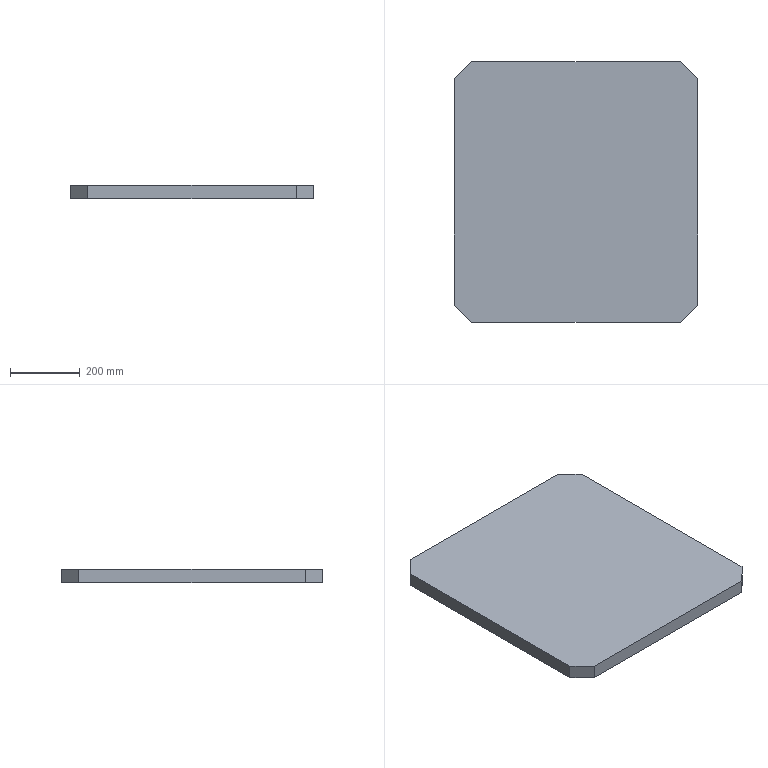Part | SolidWorks | features Extrusion 1 | 1 solid | 10 faces | box 700 x 750 x 40 mm | volume 20800000 mm3 | plane 10
STEP:
#1=CARTESIAN_POINT('',(650.,750.,0.));
#2=VERTEX_POINT('',#1);
#3=CARTESIAN_POINT('',(50.,750.,0.));
#4=VERTEX_POINT('',#3);
#5=CARTESIAN_POINT('',(50.,750.,0.));
#6=DIRECTION('',(-1.,0.,0.));
#7=VECTOR('',#6,1000.);
#8=LINE('',#5,#7);
#9=EDGE_CURVE('',#2,#4,#8,.T.);
#10=ORIENTED_EDGE('',*,*,#9,.T.);
#11=CARTESIAN_POINT('',(50.,750.,40.));
#12=VERTEX_POINT('',#11);
#13=CARTESIAN_POINT('',(50.,750.,40.));
#14=DIRECTION('',(0.,0.,-1.));
#15=VECTOR('',#14,1000.);
#16=LINE('',#13,#15);
#17=EDGE_CURVE('',#12,#4,#16,.T.);
#18=ORIENTED_EDGE('',*,*,#17,.F.);
#19=CARTESIAN_POINT('',(650.,750.,40.));
#20=VERTEX_POINT('',#19);
#21=CARTESIAN_POINT('',(50.,750.,40.));
#22=DIRECTION('',(-1.,0.,0.));
#23=VECTOR('',#22,1000.);
#24=LINE('',#21,#23);
#25=EDGE_CURVE('',#20,#12,#24,.T.);
#26=ORIENTED_EDGE('',*,*,#25,.F.);
#27=CARTESIAN_POINT('',(650.,750.,40.));
#28=DIRECTION('',(0.,0.,-1.));
#29=VECTOR('',#28,1000.);
#30=LINE('',#27,#29);
#31=EDGE_CURVE('',#20,#2,#30,.T.);
#32=ORIENTED_EDGE('',*,*,#31,.T.);
#33=EDGE_LOOP('',(#10,#18,#26,#32));
#34=FACE_OUTER_BOUND('',#33,.T.);
#35=CARTESIAN_POINT('',(50.,750.,40.));
#36=DIRECTION('',(0.,-1.,0.));
#37=DIRECTION('',(0.,0.,-1.));
#38=AXIS2_PLACEMENT_3D('',#35,#36,#37);
#39=PLANE('',#38);
#40=ADVANCED_FACE('',(#34),#39,.F.);
#41=CARTESIAN_POINT('',(0.,700.,0.));
#42=VERTEX_POINT('',#41);
#43=CARTESIAN_POINT('',(0.,700.,0.));
#44=DIRECTION('',(-0.7071,-0.7071,0.));
#45=VECTOR('',#44,1000.);
#46=LINE('',#43,#45);
#47=EDGE_CURVE('',#4,#42,#46,.T.);
#48=ORIENTED_EDGE('',*,*,#47,.T.);
#49=CARTESIAN_POINT('',(0.,700.,40.));
#50=VERTEX_POINT('',#49);
#51=CARTESIAN_POINT('',(0.,700.,40.));
#52=DIRECTION('',(0.,0.,-1.));
#53=VECTOR('',#52,1000.);
#54=LINE('',#51,#53);
#55=EDGE_CURVE('',#50,#42,#54,.T.);
#56=ORIENTED_EDGE('',*,*,#55,.F.);
#57=CARTESIAN_POINT('',(0.,700.,40.));
#58=DIRECTION('',(-0.7071,-0.7071,0.));
#59=VECTOR('',#58,1000.);
#60=LINE('',#57,#59);
#61=EDGE_CURVE('',#12,#50,#60,.T.);
#62=ORIENTED_EDGE('',*,*,#61,.F.);
#63=ORIENTED_EDGE('',*,*,#17,.T.);
#64=EDGE_LOOP('',(#48,#56,#62,#63));
#65=FACE_OUTER_BOUND('',#64,.T.);
#66=CARTESIAN_POINT('',(0.,700.,40.));
#67=DIRECTION('',(0.7071,-0.7071,0.));
#68=DIRECTION('',(0.7071,0.7071,0.));
#69=AXIS2_PLACEMENT_3D('',#66,#67,#68);
#70=PLANE('',#69);
#71=ADVANCED_FACE('',(#65),#70,.F.);
#72=CARTESIAN_POINT('',(0.,50.,0.));
#73=VERTEX_POINT('',#72);
#74=CARTESIAN_POINT('',(0.,50.,0.));
#75=DIRECTION('',(0.,-1.,0.));
#76=VECTOR('',#75,1000.);
#77=LINE('',#74,#76);
#78=EDGE_CURVE('',#42,#73,#77,.T.);
#79=ORIENTED_EDGE('',*,*,#78,.T.);
#80=CARTESIAN_POINT('',(0.,50.,40.));
#81=VERTEX_POINT('',#80);
#82=CARTESIAN_POINT('',(0.,50.,40.));
#83=DIRECTION('',(0.,0.,-1.));
#84=VECTOR('',#83,1000.);
#85=LINE('',#82,#84);
#86=EDGE_CURVE('',#81,#73,#85,.T.);
#87=ORIENTED_EDGE('',*,*,#86,.F.);
#88=CARTESIAN_POINT('',(0.,50.,40.));
#89=DIRECTION('',(0.,-1.,0.));
#90=VECTOR('',#89,1000.);
#91=LINE('',#88,#90);
#92=EDGE_CURVE('',#50,#81,#91,.T.);
#93=ORIENTED_EDGE('',*,*,#92,.F.);
#94=ORIENTED_EDGE('',*,*,#55,.T.);
#95=EDGE_LOOP('',(#79,#87,#93,#94));
#96=FACE_OUTER_BOUND('',#95,.T.);
#97=CARTESIAN_POINT('',(0.,50.,40.));
#98=DIRECTION('',(1.,0.,0.));
#99=DIRECTION('',(0.,0.,-1.));
#100=AXIS2_PLACEMENT_3D('',#97,#98,#99);
#101=PLANE('',#100);
#102=ADVANCED_FACE('',(#96),#101,.F.);
#103=CARTESIAN_POINT('',(50.,0.,0.));
#104=VERTEX_POINT('',#103);
#105=CARTESIAN_POINT('',(50.,0.,0.));
#106=DIRECTION('',(0.7071,-0.7071,0.));
#107=VECTOR('',#106,1000.);
#108=LINE('',#105,#107);
#109=EDGE_CURVE('',#73,#104,#108,.T.);
#110=ORIENTED_EDGE('',*,*,#109,.T.);
#111=CARTESIAN_POINT('',(50.,0.,40.));
#112=VERTEX_POINT('',#111);
#113=CARTESIAN_POINT('',(50.,0.,40.));
#114=DIRECTION('',(0.,0.,-1.));
#115=VECTOR('',#114,1000.);
#116=LINE('',#113,#115);
#117=EDGE_CURVE('',#112,#104,#116,.T.);
#118=ORIENTED_EDGE('',*,*,#117,.F.);
#119=CARTESIAN_POINT('',(50.,0.,40.));
#120=DIRECTION('',(0.7071,-0.7071,0.));
#121=VECTOR('',#120,1000.);
#122=LINE('',#119,#121);
#123=EDGE_CURVE('',#81,#112,#122,.T.);
#124=ORIENTED_EDGE('',*,*,#123,.F.);
#125=ORIENTED_EDGE('',*,*,#86,.T.);
#126=EDGE_LOOP('',(#110,#118,#124,#125));
#127=FACE_OUTER_BOUND('',#126,.T.);
#128=CARTESIAN_POINT('',(50.,0.,40.));
#129=DIRECTION('',(0.7071,0.7071,0.));
#130=DIRECTION('',(-0.7071,0.7071,0.));
#131=AXIS2_PLACEMENT_3D('',#128,#129,#130);
#132=PLANE('',#131);
#133=ADVANCED_FACE('',(#127),#132,.F.);
#134=CARTESIAN_POINT('',(650.,0.,0.));
#135=VERTEX_POINT('',#134);
#136=CARTESIAN_POINT('',(50.,0.,0.));
#137=DIRECTION('',(1.,0.,0.));
#138=VECTOR('',#137,1000.);
#139=LINE('',#136,#138);
#140=EDGE_CURVE('',#104,#135,#139,.T.);
#141=ORIENTED_EDGE('',*,*,#140,.T.);
#142=CARTESIAN_POINT('',(650.,0.,40.));
#143=VERTEX_POINT('',#142);
#144=CARTESIAN_POINT('',(650.,0.,40.));
#145=DIRECTION('',(0.,0.,-1.));
#146=VECTOR('',#145,1000.);
#147=LINE('',#144,#146);
#148=EDGE_CURVE('',#143,#135,#147,.T.);
#149=ORIENTED_EDGE('',*,*,#148,.F.);
#150=CARTESIAN_POINT('',(50.,0.,40.));
#151=DIRECTION('',(1.,0.,0.));
#152=VECTOR('',#151,1000.);
#153=LINE('',#150,#152);
#154=EDGE_CURVE('',#112,#143,#153,.T.);
#155=ORIENTED_EDGE('',*,*,#154,.F.);
#156=ORIENTED_EDGE('',*,*,#117,.T.);
#157=EDGE_LOOP('',(#141,#149,#155,#156));
#158=FACE_OUTER_BOUND('',#157,.T.);
#159=CARTESIAN_POINT('',(50.,0.,40.));
#160=DIRECTION('',(0.,1.,0.));
#161=DIRECTION('',(0.,0.,1.));
#162=AXIS2_PLACEMENT_3D('',#159,#160,#161);
#163=PLANE('',#162);
#164=ADVANCED_FACE('',(#158),#163,.F.);
#165=CARTESIAN_POINT('',(700.,50.,0.));
#166=VERTEX_POINT('',#165);
#167=CARTESIAN_POINT('',(650.,0.,0.));
#168=DIRECTION('',(0.7071,0.7071,0.));
#169=VECTOR('',#168,1000.);
#170=LINE('',#167,#169);
#171=EDGE_CURVE('',#135,#166,#170,.T.);
#172=ORIENTED_EDGE('',*,*,#171,.T.);
#173=CARTESIAN_POINT('',(700.,50.,40.));
#174=VERTEX_POINT('',#173);
#175=CARTESIAN_POINT('',(700.,50.,40.));
#176=DIRECTION('',(0.,0.,-1.));
#177=VECTOR('',#176,1000.);
#178=LINE('',#175,#177);
#179=EDGE_CURVE('',#174,#166,#178,.T.);
#180=ORIENTED_EDGE('',*,*,#179,.F.);
#181=CARTESIAN_POINT('',(650.,0.,40.));
#182=DIRECTION('',(0.7071,0.7071,0.));
#183=VECTOR('',#182,1000.);
#184=LINE('',#181,#183);
#185=EDGE_CURVE('',#143,#174,#184,.T.);
#186=ORIENTED_EDGE('',*,*,#185,.F.);
#187=ORIENTED_EDGE('',*,*,#148,.T.);
#188=EDGE_LOOP('',(#172,#180,#186,#187));
#189=FACE_OUTER_BOUND('',#188,.T.);
#190=CARTESIAN_POINT('',(650.,0.,40.));
#191=DIRECTION('',(-0.7071,0.7071,0.));
#192=DIRECTION('',(-0.7071,-0.7071,0.));
#193=AXIS2_PLACEMENT_3D('',#190,#191,#192);
#194=PLANE('',#193);
#195=ADVANCED_FACE('',(#189),#194,.F.);
#196=CARTESIAN_POINT('',(700.,700.,0.));
#197=VERTEX_POINT('',#196);
#198=CARTESIAN_POINT('',(700.,50.,0.));
#199=DIRECTION('',(0.,1.,0.));
#200=VECTOR('',#199,1000.);
#201=LINE('',#198,#200);
#202=EDGE_CURVE('',#166,#197,#201,.T.);
#203=ORIENTED_EDGE('',*,*,#202,.T.);
#204=CARTESIAN_POINT('',(700.,700.,40.));
#205=VERTEX_POINT('',#204);
#206=CARTESIAN_POINT('',(700.,700.,40.));
#207=DIRECTION('',(0.,0.,-1.));
#208=VECTOR('',#207,1000.);
#209=LINE('',#206,#208);
#210=EDGE_CURVE('',#205,#197,#209,.T.);
#211=ORIENTED_EDGE('',*,*,#210,.F.);
#212=CARTESIAN_POINT('',(700.,50.,40.));
#213=DIRECTION('',(0.,1.,0.));
#214=VECTOR('',#213,1000.);
#215=LINE('',#212,#214);
#216=EDGE_CURVE('',#174,#205,#215,.T.);
#217=ORIENTED_EDGE('',*,*,#216,.F.);
#218=ORIENTED_EDGE('',*,*,#179,.T.);
#219=EDGE_LOOP('',(#203,#211,#217,#218));
#220=FACE_OUTER_BOUND('',#219,.T.);
#221=CARTESIAN_POINT('',(700.,50.,40.));
#222=DIRECTION('',(-1.,0.,0.));
#223=DIRECTION('',(0.,0.,1.));
#224=AXIS2_PLACEMENT_3D('',#221,#222,#223);
#225=PLANE('',#224);
#226=ADVANCED_FACE('',(#220),#225,.F.);
#227=CARTESIAN_POINT('',(650.,750.,0.));
#228=DIRECTION('',(-0.7071,0.7071,0.));
#229=VECTOR('',#228,1000.);
#230=LINE('',#227,#229);
#231=EDGE_CURVE('',#197,#2,#230,.T.);
#232=ORIENTED_EDGE('',*,*,#231,.T.);
#233=ORIENTED_EDGE('',*,*,#31,.F.);
#234=CARTESIAN_POINT('',(650.,750.,40.));
#235=DIRECTION('',(-0.7071,0.7071,0.));
#236=VECTOR('',#235,1000.);
#237=LINE('',#234,#236);
#238=EDGE_CURVE('',#205,#20,#237,.T.);
#239=ORIENTED_EDGE('',*,*,#238,.F.);
#240=ORIENTED_EDGE('',*,*,#210,.T.);
#241=EDGE_LOOP('',(#232,#233,#239,#240));
#242=FACE_OUTER_BOUND('',#241,.T.);
#243=CARTESIAN_POINT('',(650.,750.,40.));
#244=DIRECTION('',(-0.7071,-0.7071,0.));
#245=DIRECTION('',(0.7071,-0.7071,0.));
#246=AXIS2_PLACEMENT_3D('',#243,#244,#245);
#247=PLANE('',#246);
#248=ADVANCED_FACE('',(#242),#247,.F.);
#249=ORIENTED_EDGE('',*,*,#25,.T.);
#250=ORIENTED_EDGE('',*,*,#61,.T.);
#251=ORIENTED_EDGE('',*,*,#92,.T.);
#252=ORIENTED_EDGE('',*,*,#123,.T.);
#253=ORIENTED_EDGE('',*,*,#154,.T.);
#254=ORIENTED_EDGE('',*,*,#185,.T.);
#255=ORIENTED_EDGE('',*,*,#216,.T.);
#256=ORIENTED_EDGE('',*,*,#238,.T.);
#257=EDGE_LOOP('',(#249,#250,#251,#252,#253,#254,#255,#256));
#258=FACE_OUTER_BOUND('',#257,.T.);
#259=CARTESIAN_POINT('',(700.,750.,40.));
#260=DIRECTION('',(0.,0.,1.));
#261=DIRECTION('',(1.,0.,0.));
#262=AXIS2_PLACEMENT_3D('',#259,#260,#261);
#263=PLANE('',#262);
#264=ADVANCED_FACE('',(#258),#263,.T.);
#265=ORIENTED_EDGE('',*,*,#9,.F.);
#266=ORIENTED_EDGE('',*,*,#231,.F.);
#267=ORIENTED_EDGE('',*,*,#202,.F.);
#268=ORIENTED_EDGE('',*,*,#171,.F.);
#269=ORIENTED_EDGE('',*,*,#140,.F.);
#270=ORIENTED_EDGE('',*,*,#109,.F.);
#271=ORIENTED_EDGE('',*,*,#78,.F.);
#272=ORIENTED_EDGE('',*,*,#47,.F.);
#273=EDGE_LOOP('',(#265,#266,#267,#268,#269,#270,#271,#272));
#274=FACE_OUTER_BOUND('',#273,.T.);
#275=CARTESIAN_POINT('',(700.,750.,0.));
#276=DIRECTION('',(0.,0.,1.));
#277=DIRECTION('',(1.,0.,0.));
#278=AXIS2_PLACEMENT_3D('',#275,#276,#277);
#279=PLANE('',#278);
#280=ADVANCED_FACE('',(#274),#279,.F.);
#281=CLOSED_SHELL('',(#40,#71,#102,#133,#164,#195,#226,#248,#264,#280));
#282=MANIFOLD_SOLID_BREP('',#281);
#283=CARTESIAN_POINT('',(0.,0.,0.));
#284=DIRECTION('',(0.,0.,1.));
#285=DIRECTION('',(1.,0.,0.));
#286=AXIS2_PLACEMENT_3D('',#283,#284,#285);
#287=(LENGTH_UNIT()NAMED_UNIT(*)SI_UNIT(.MILLI.,.METRE.));
#288=UNCERTAINTY_MEASURE_WITH_UNIT(LENGTH_MEASURE(0.00001),#287,'','');
#289=(NAMED_UNIT(*)PLANE_ANGLE_UNIT()SI_UNIT($,.RADIAN.));
#290=(NAMED_UNIT(*)SI_UNIT($,.STERADIAN.)SOLID_ANGLE_UNIT());
#291=(GEOMETRIC_REPRESENTATION_CONTEXT(3)GLOBAL_UNCERTAINTY_ASSIGNED_CONTEXT((#288))GLOBAL_UNIT_ASSIGNED_CONTEXT((#287,#289,#290))REPRESENTATION_CONTEXT('',''));
#292=ADVANCED_BREP_SHAPE_REPRESENTATION('',(#282,#286),#291);